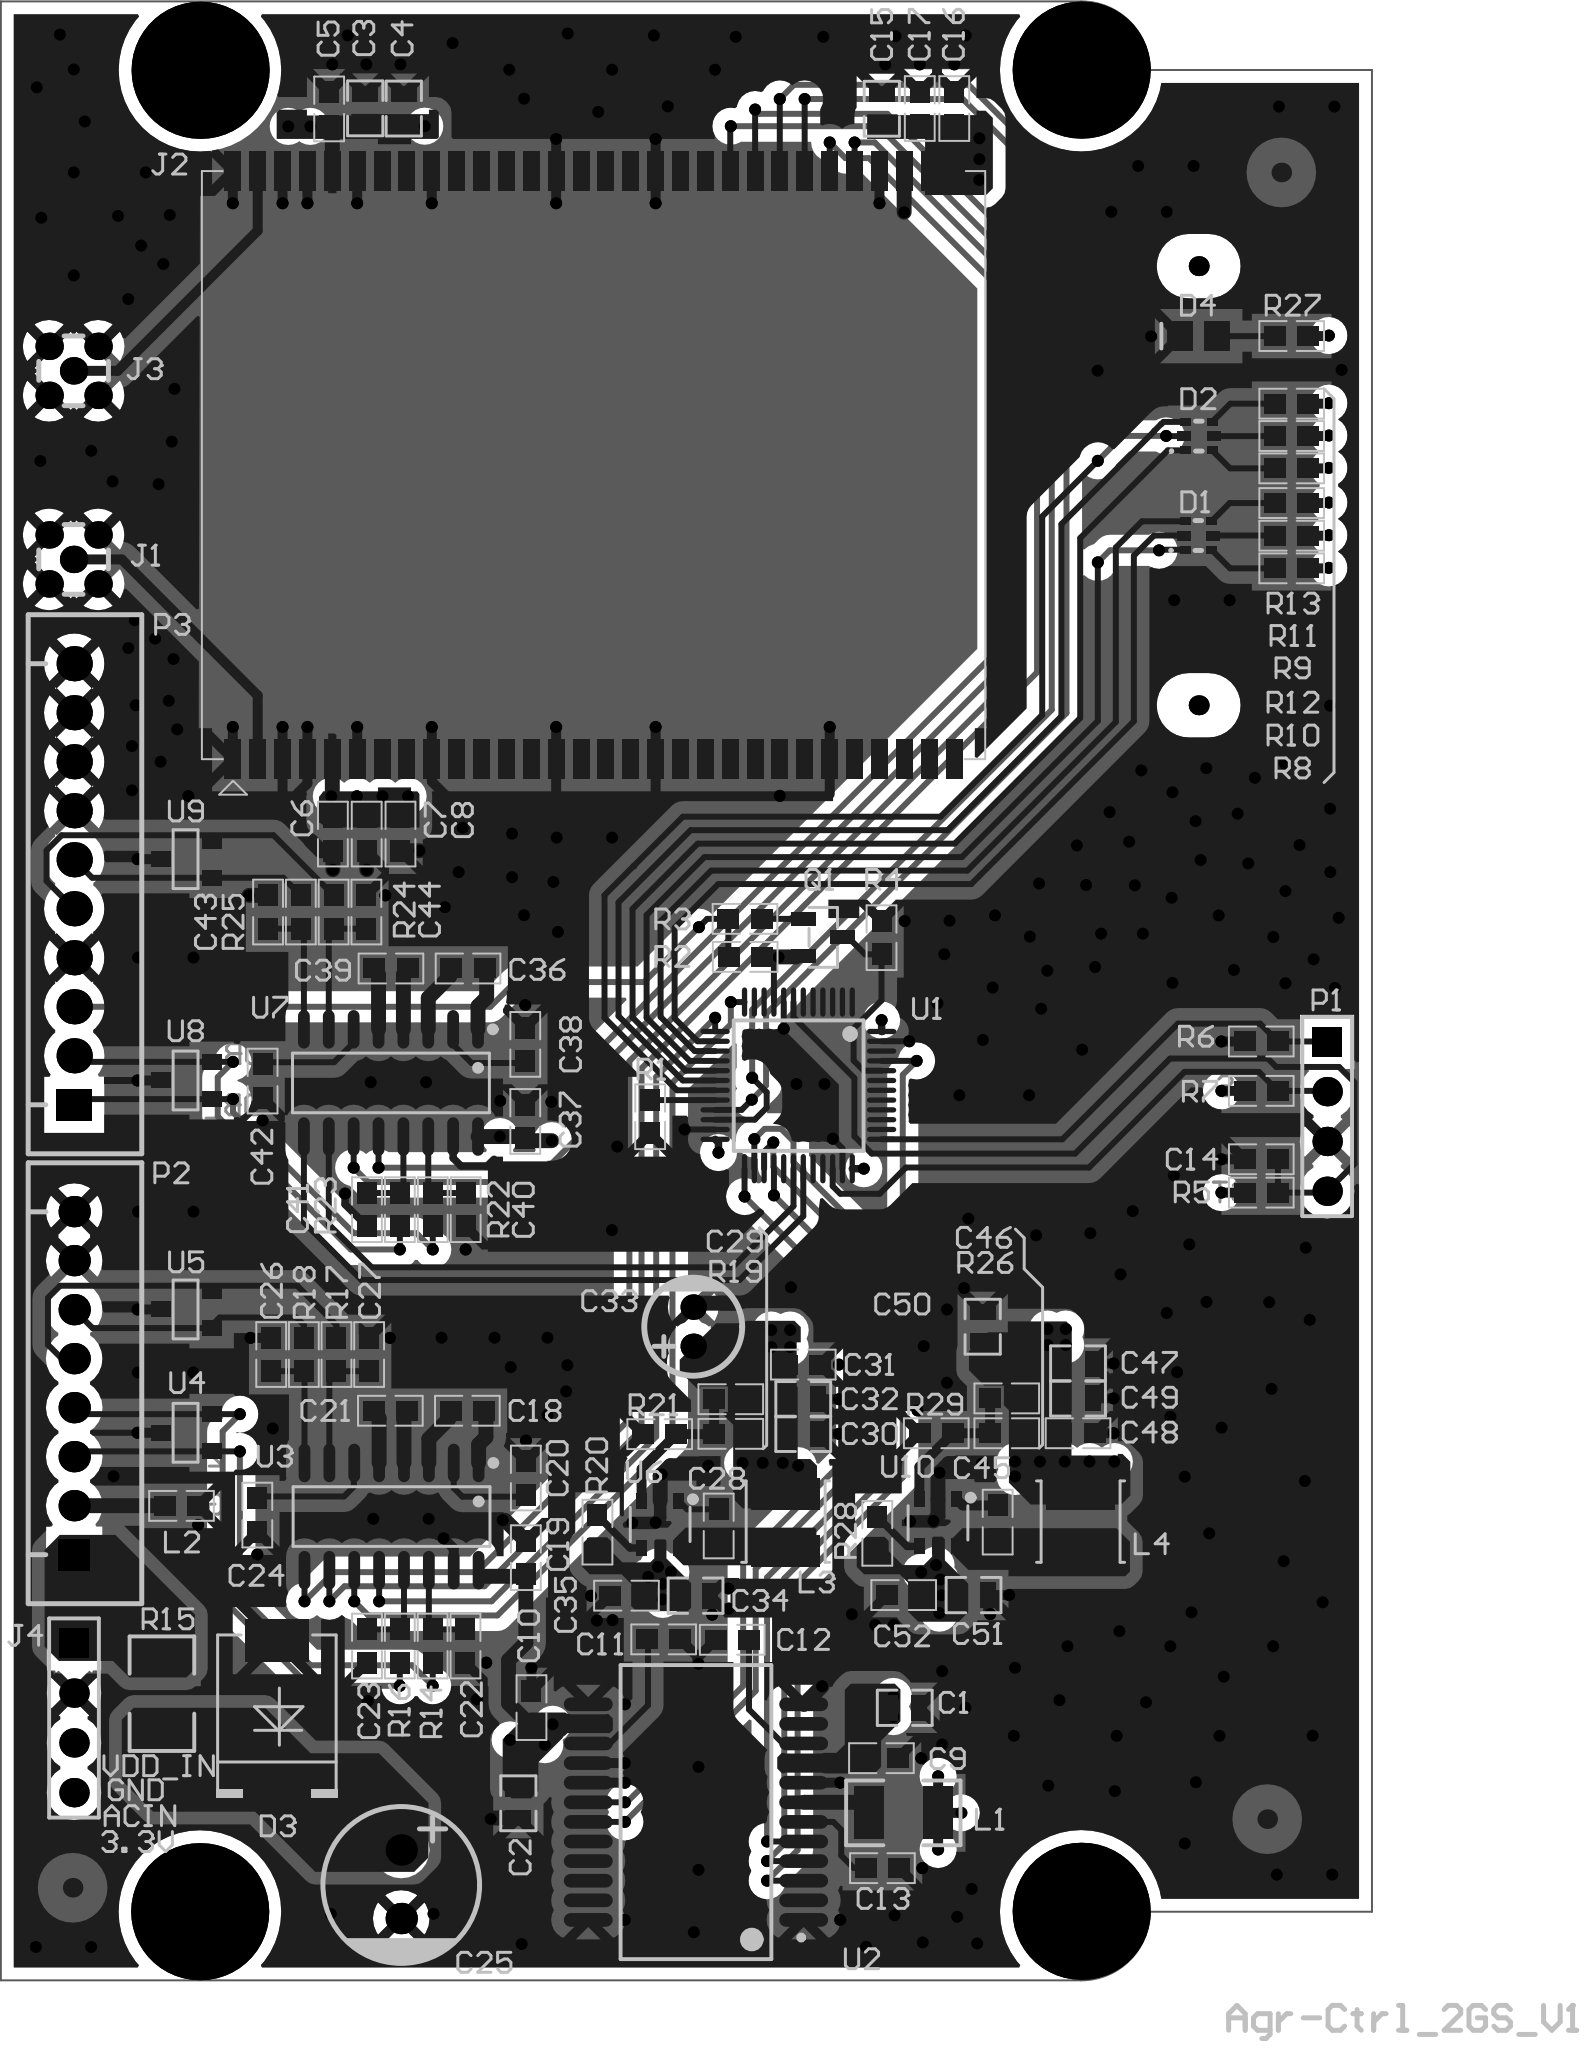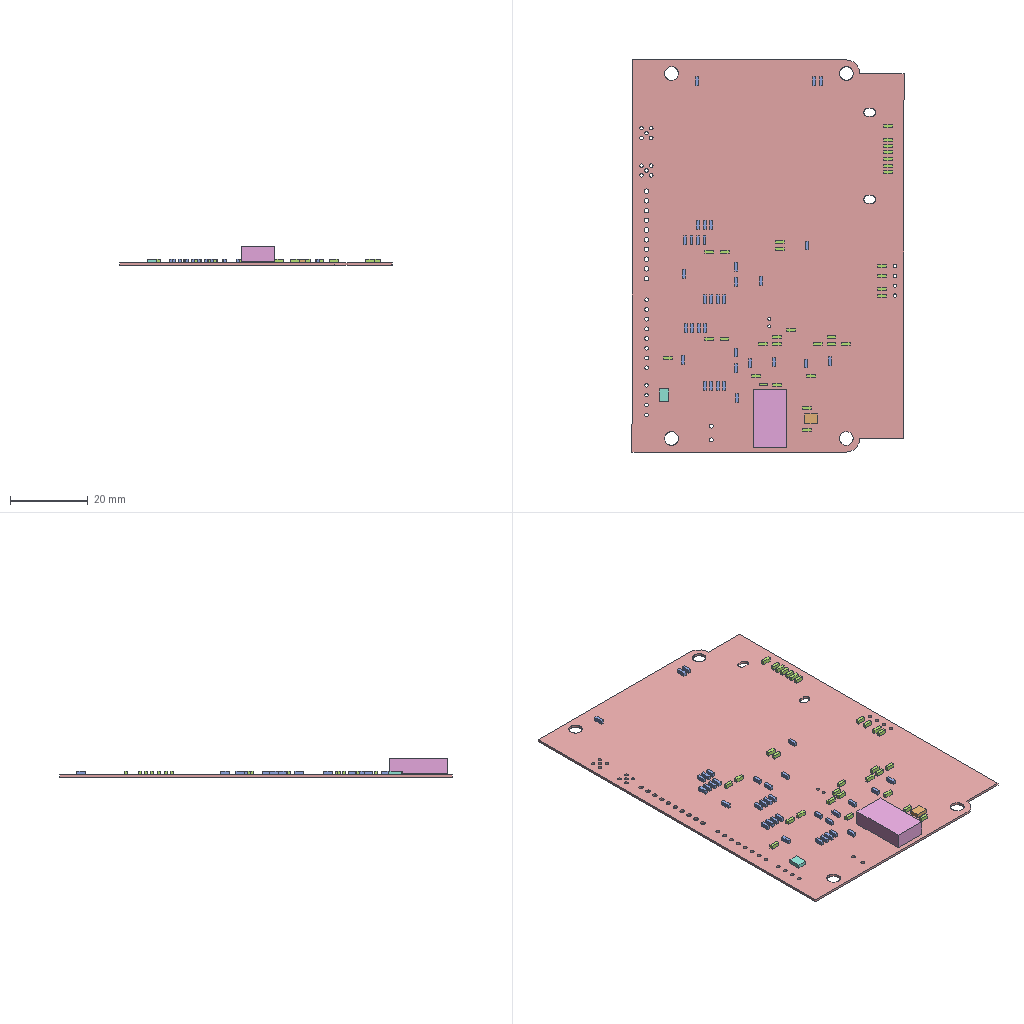Circuit board layout | Altium Designer | box 70 x 100.9 x 4.8 mm
Layer stack:
# Altium Designer layer stack of  (unit mm; dielectric type: 0 none, 1 core, 2 prepreg, 3 surface material)
index,name,kind,layer,copper_thickness_mm,dielectric_type,dielectric_thickness_mm,dielectric_material,dielectric_constant
0,Top Paste,other,,,,,,
1,Top Overlay,other,,,,,,
2,Top Solder,dielectric,,,3,0.0102,Solder Resist,3.5
3,Top Layer,copper,Top Layer,0.0356,,,,
4,Dielectric1,dielectric,,,2,0.0711,PP-006,4.1
5,GND2,copper,GND2,0.035,,,,
6,Dielectric5,dielectric,,,0,0.32,FR-4,4.8
7,POWER3,copper,POWER3,0.035,,,,
8,Dielectric6,dielectric,,,2,0.0711,PP-006,4.1
9,Bottom Layer,copper,Bottom Layer,0.0356,,,,
10,Bottom Solder,dielectric,,,3,0.0102,Solder Resist,3.5
11,Bottom Overlay,other,,,,,,
12,Bottom Paste,other,,,,,,
# drill layer pairs: low layer,high layer
drill_pair,Top Layer,Bottom Layer
Part placement:
Designator,Comment,Layer,Footprint,Center-X(mm),Center-Y(mm),Rotation
U5,PESD15VL2BT,TopLayer,SOT-23,78.797,84,90
P1,Header,TopLayer,HDR1X4,137.06,93.84,270
U7,SP3232EEN,TopLayer,SOP16-6.6,89.255,95.555,270
C41,15pF/50V,TopLayer,0603,88.029,89.09,90
R25,4.7O,±1%,TopLayer,0603,84.653,104.273,270
R24,4.7O,±1%,TopLayer,0603,86.327,104.273,270
R23,4.7O,±1%,TopLayer,0603,89.71,89.09,90
R22,4.7O,±1%,TopLayer,0603,91.39,89.09,90
R21,10K,TopLayer,0603,102.978,77.639,360
R20,100K,TopLayer,0603,99.8,72.64,270
R19,75K 1%,TopLayer,0603,106.608,77.655,360
R18,4.7O,±1%,TopLayer,0603,84.807,81.7,270
R6,10K,TopLayer,0603,133.696,97.67,180
D3,SMCJ18A,TopLayer,SMC_L6.9-W5.9-LS7.9-RD,83.43,63.42,90
C1,22uF/10V,TopLayer,C0805,115.49,63.68,360
C2,22uF/10V,TopLayer,C0805,95.76,58.809,270
C3,10uF/25V,TopLayer,C0805,87.94,145.27,270
C4,10uF/25V,TopLayer,C0805,89.91,145.26,270
C5,100nF/50V,TopLayer,0603,86.1,145.24,90
C6,100pF/50V,TopLayer,0603,86.29,108.25,270
C7,100pF/50V,TopLayer,0603,88.016,108.25,90
C8,100nF/50V,TopLayer,0603,89.741,108.25,90
C9,1uF/25V,TopLayer,0603,114.3,61.11,360
C10,100nF/50V,TopLayer,0603,96.43,63.69,90
C11,1uF/25V,TopLayer,0603,103.18,67.17,360
C12,1uF/25V,TopLayer,0603,106.68,67.15,180
C13,470nF/50V,TopLayer,0603,114.35,55.5,360
C15,10uF/25V,TopLayer,C0805,114.32,145.25,270
C16,100pF/50V,TopLayer,0603,118.02,145.26,270
C17,100nF/50V,TopLayer,0603,116.257,145.26,270
C25,470uF/25V,TopLayer,CAP-TH_BD8.0-P3.50-D1.0-FD,89.78,54.68,270
C28,100nF/50V,TopLayer,0603,105.99,72.956,90
C29,100pF/50V,TopLayer,0603,106.608,79.421,180
C30,22uF/10V,TopLayer,C0805,110.308,77.655,360
C31,100nF/50V,TopLayer,0603,110.308,81.186,360
C32,22uF/10V,TopLayer,C0805,110.308,79.421,360
C33,100uF/10V,TopLayer,CAP-TH_BD5.0-P2.00-D0.8-FD,104.69,83.12,90
C34,10uF/25V,TopLayer,C0805,104.808,69.4,180
C35,100nF/50V,TopLayer,0603,101.28,69.4,360
C39,100nF/50V,TopLayer,0603,89.255,101.392,360
C45,100nF/50V,TopLayer,0603,120.236,73.152,90
C46,100pF/50V,TopLayer,0603,120.7,79.463,180
C47,22uF/10V,TopLayer,C0805,124.339,81.241,360
C48,100nF/50V,TopLayer,0603,124.339,77.685,360
C49,22uF/10V,TopLayer,C0805,124.339,79.463,360
C50,22uF/10V,TopLayer,C0805,119.47,83.12,90
C51,10uF/25V,TopLayer,C0805,119.004,69.43,180
C52,100nF/50V,TopLayer,0603,115.437,69.43,360
D1,Full-color RGB LED,TopLayer,RGB,130.48,123.48,180
D2,Full-color RGB LED,TopLayer,RGB,130.51,128.55,180
D4,RED,TopLayer,LED_0805,130.5,133.65,180
J2,UM482/K823,TopLayer,UM482/K823,99.595,127.07,90
L2,120O ±25% @100MHz,TopLayer,0603,78.56,73.98,360
L3,2.2uH/2A,TopLayer,IND-SMD_L4.0-W4.0,109.41,73.15,90
L4,2.2uH/2A,TopLayer,IND-SMD_L4.0-W4.0,124.47,73.15,90
P2,XH-8A,TopLayer,CONN-TH_XH-8A,73.08,80.24,90
P3,XH-10A,TopLayer,CONN-TH_10P-P2.50_XH-10A,73.08,105.69,90
Q1,8550,TopLayer,SOT-23-SS8550,111.33,102.98,180
R11,680R,TopLayer,0603,135.25,128.555,180
R12,1K,TopLayer,0603,135.25,125.135,180
R13,1K,TopLayer,0603,135.25,130.205,180
R26,100K,TopLayer,0603,120.7,77.685,360
R27,1K,TopLayer,0603,135.25,133.655,360
R28,100K,TopLayer,0603,114.09,72.58,270
R29,22.1K,TopLayer,0603,117.1,77.685,360
U1,STM32F103C8T6/GD32F103C8T6,TopLayer,LQFP-48_L7.0-W7.0-P0.50-LS9.0-BL,110.06,95.43,180
U2,SCC2130,TopLayer,SCC2130D,104.83,58.36,180
U3,SP3232EEN,TopLayer,SOP16-6.6,89.285,73.436,270
U4,PESD15VL2BT,TopLayer,SOT-23,78.797,77.71,90
U8,PESD15VL2BT,TopLayer,SOT-23,78.797,95.68,90
U9,PESD15VL2BT,TopLayer,SOT-23,78.797,106.97,90
R1,10K,TopLayer,0603,102.49,93.83,90
R2,10K,TopLayer,0603,107.344,101.984,360
R4,10K,TopLayer,0603,114.304,102.964,270
R5,10K,TopLayer,0603,133.696,89.96,180
R7,10K,TopLayer,0603,133.696,95.15,180
R8,1.5K,TopLayer,0603,135.25,121.805,180
R9,1.5K,TopLayer,0603,135.25,126.905,180
R10,680R,TopLayer,0603,135.25,123.47,180
R14,4.7O,±1%,TopLayer,0603,91.383,66.831,90
R15,12V/2A,TopLayer,1210,77.56,64.4,90
R16,4.7O,±1%,TopLayer,0603,89.707,66.831,90
R17,4.7O,±1%,TopLayer,0603,86.473,81.7,270
C18,100nF/50V,TopLayer,0603,93.156,78.833,360
C19,100nF/50V,TopLayer,0603,96.143,71.338,90
C20,100nF/50V,TopLayer,0603,96.143,75.401,90
C21,100nF/50V,TopLayer,0603,89.224,78.833,360
C22,15pF/50V,TopLayer,0603,93.06,66.831,90
C23,15pF/50V,TopLayer,0603,88.03,66.831,90
C24,100nF/50V,TopLayer,0603,82.431,73.511,270
C26,15pF/50V,TopLayer,0603,83.14,81.7,90
C27,15pF/50V,TopLayer,0603,88.14,81.7,90
C36,100nF/50V,TopLayer,0603,93.192,101.392,360
C37,100nF/50V,TopLayer,0603,96.113,93.59,90
C38,100nF/50V,TopLayer,0603,96.113,97.522,90
C40,15pF/50V,TopLayer,0603,93.07,89.09,90
C42,100nF/50V,TopLayer,0603,82.7,95.65,270
C43,15pF/50V,TopLayer,0603,82.98,104.273,90
C44,15pF/50V,TopLayer,0603,88,104.273,90
C14,100nF/50V,TopLayer,0603,133.696,91.66,360
L1,47uH±20%,TopLayer,1210,115.418,58.32,180
R3,10K,TopLayer,0603,107.334,103.924,180
J1,MMCX-KE RF connector,TopLayer,MMCX-TH_ZC11.801KK,73.05,122.26,180
J3,MMCX-KE RF connector,TopLayer,MMCX-TH_ZC11.801KK,73.05,131.88,360
J4,Header,TopLayer,HDR1X4,73.07,63.16,270
U6,SY8113B,TopLayer,TSOT-23-6_L2.9-W1.6-P0.95-LS2.8-BR,103.002,73.033,90
U10,SY8113B,TopLayer,TSOT-23-6_L2.9-W1.6-P0.95-LS2.8-BR,117.188,73.113,90
Pad and via stacks:
# Altium Designer via and pad stacks of  (unit mm). Each distinct definition once, with the count of objects using it.
# via: kind,start_layer,end_layer,hole_mm,diameter_mm,mode(0 simple;1 top-mid-bottom;2 full stack),diameter_per_layer,count,example_net
# pad: kind,layer,hole_mm,hole_type(0 round;1 square;2 slot),plating,top_size,top_shape(1 round;2 rect;3 octagon;9 rounded rect),mid_size,bottom_size,mode,footprint,size_per_layer,count,example
pad,Top Layer,0,0,plated,0.8x1,2,0.8x1,0.8x1,0,SOT-23,,12,U9.2
pad,Top Layer,0,0,plated,1.6x3.5,2,1.6x3.5,1.6x3.5,0,IND-SMD_L4.0-W4.0,,4,L4.2
pad,Top Layer,0,0,plated,1.3x0.8,2,1.3x0.8,1.3x0.8,0,C0805,,24,C2.2
pad,Top Layer,0,0,plated,1x1.1,2,1x1.1,1x1.1,0,0603,,134,C42.2
pad,Top Layer,0,0,plated,2.158x3.24,2,2.158x3.24,2.158x3.24,0,SMC_L6.9-W5.9-LS7.9-RD,,2,D3.2
pad,Top Layer,0,0,plated,0.8x0.532,2,0.8x0.532,0.8x0.532,0,TSOT-23-6_L2.9-W1.6-P0.95-LS2.8-BR,,12,U10.1
pad,Top Layer,0,0,plated,1.25x0.7,2,1.25x0.7,1.25x0.7,0,SOT-23-SS8550,,3,Q1.1
pad,Top Layer,0,0,plated,1x1,1,1x1,1x1,0,,,3,MARK
pad,Top Layer,0,0,plated,2.01x0.85,2,2.01x0.85,2.01x0.85,0,UM482/K823,,60,J2.30
pad,Top Layer,0,0,plated,0.602x1.971,1,0.602x1.971,0.602x1.971,0,SOP16-6.6,,32,U7.9
pad,Top Layer,0,0,plated,1.524x2.7,2,1.524x2.7,1.524x2.7,0,1210,,4,L1.1
pad,Top Layer,0,0,plated,0.7x2.5,1,0.7x2.5,0.7x2.5,0,SCC2130D,,24,U2.13
pad,Top Layer,0,0,plated,0.27x1.5,1,0.27x1.5,0.27x1.5,0,LQFP-48_L7.0-W7.0-P0.50-LS9.0-BL,,24,U1.1
pad,Top Layer,0,0,plated,1.5x0.27,1,1.5x0.27,1.5x0.27,0,LQFP-48_L7.0-W7.0-P0.50-LS9.0-BL,,24,U1.13
pad,Top Layer,0,0,plated,0.55x0.4,2,0.55x0.4,0.55x0.4,0,RGB,,8,D1.1
pad,Top Layer,0,0,plated,0.7x0.5,2,0.7x0.5,0.7x0.5,0,RGB,,4,D1.3
pad,Top Layer,0,0,plated,1.5x1.3,2,1.5x1.3,1.5x1.3,0,LED_0805,,2,D4.2
pad,Multi-Layer,0.8,0,plated,1.3x1.3,1,1.3x1.3,1.3x1.3,0,CAP-TH_BD5.0-P2.00-D0.8-FD,,2,C33.1
pad,Multi-Layer,2,2,unplated,1.016x1.016,1,1.016x1.016,1.016x1.016,0,,,2,0
pad,Multi-Layer,0.9,0,plated,1.5x1.5,2,1.5x1.5,1.5x1.5,0,HDR1X4,,2,P1.1
pad,Multi-Layer,0.9,0,plated,1.5x1.5,1,1.5x1.5,1.5x1.5,0,HDR1X4,,6,P1.2
pad,Multi-Layer,1,0,plated,1.6x1.6,1,1.6x1.6,1.6x1.6,0,CAP-TH_BD8.0-P3.50-D1.0-FD,,2,C25.2
pad,Multi-Layer,0.9,0,plated,1.4x1.4,1,1.4x1.4,1.4x1.4,0,MMCX-TH_ZC11.801KK,,10,J3.5
pad,Multi-Layer,1.2,0,plated,1.8x1.8,1,1.8x1.8,1.8x1.8,0,CONN-TH_10P-P2.50_XH-10A,,9,P3.10
pad,Multi-Layer,1.2,0,plated,1.6x1.8,2,1.6x1.8,1.6x1.8,0,CONN-TH_10P-P2.50_XH-10A,,1,P3.1
pad,Multi-Layer,1,0,plated,1.6x1.6,1,1.6x1.6,1.6x1.6,0,CONN-TH_XH-8A,,7,P2.8
pad,Multi-Layer,1,0,plated,1.6x1.6,2,1.6x1.6,1.6x1.6,0,CONN-TH_XH-8A,,1,P2.1
pad,Multi-Layer,3.5,0,unplated,7x7,1,7x7,7x7,0,,,4,1
via,Top Layer,Bottom Layer,0.3048,0.6096,0,,390,GND
Copper pours:
name,layer,net,type(0 solid;1 hatched;2 none)
BottomLayer-No Net,Top Layer,VDD_12V,0
BottomLayer-No Net,Top Layer,VDD_12V,0
BottomLayer-No Net,Top Layer,VDD_12V,0
BottomLayer-No Net,Top Layer,VDD_IN,0
Top Layer-GND 1,Top Layer,GND,0
Top Layer-VDD_3.3,Top Layer,VDD_3.3,0
Top Layer-GND,Top Layer,GND,0
Top Layer-GND,Top Layer,GND,0
Top Layer-VDD_5V,Top Layer,VDD_5V,0
Top Layer-VDD_3.3 3,Top Layer,VDD_3.3,0
Top Layer-VDD_5V 1,Top Layer,VDD_5V,0
Top Layer-VDD_3.3 1,Top Layer,VDD_3.3,0
Top Layer-VDD_3.3 2,Top Layer,VDD_3.3,0
Top Layer-VDD_5V 2,Top Layer,VDD_5V,0
Top Layer-NetC45_1,Top Layer,NetC45_1,0
Top Layer-NetC28_1,Top Layer,NetC28_1,0
Bottom Layer-GND,Bottom Layer,GND,0
Design rules, without the lines most boards share:
# Altium Designer design rules of  (exported by Altium Designer, unit mm)
# columns: name | kind | enabled | priority | scope1 | scope2 | descriptor | typed fields (field=value)
PolygonConnect_1 | 20 | enabled | 1 | ISVIA | All | Polygon Connect Rule(Direct Connect )(Conductor Width=10mil) (Relief Angle=90 Angle) (Entries=4) (Air Gap Width=10mil) (ISVIA),(All) | connect_style(0=relief,1=direct,2=none)=1 relief_conductor_width=0.254 relief_entries=4
Clearance | 0 | enabled | 3 | All | All | Clearance Constraint (Gap=6mil) (All),(All) | gap=0.1524
mark | 0 | enabled | 1 | HASPAD('FREE-MARK') | All | Clearance Constraint (Gap=50mil) (HASPAD('FREE-MARK')),(All) | gap=1.27
PolygonConnect | 20 | enabled | 3 | All | All | Polygon Connect Rule(Direct Connect )(Conductor Width=10mil) (Relief Angle=90 Angle) (Entries=4) (Air Gap Width=10mil) (All),(All) | connect_style(0=relief,1=direct,2=none)=1 relief_conductor_width=0.254 relief_entries=4
PolygonGND | 20 | enabled | 2 | InNet('GND') | All | Polygon Connect Rule(Relief Connect )(Conductor Width=20mil) (Relief Angle=45 Angle) (Entries=4) (Air Gap Width=10mil) (InNet('GND')),(All) | connect_style(0=relief,1=direct,2=none)=0 relief_conductor_width=0.508 relief_entries=4
GND_Clearance | 0 | enabled | 2 | InNet('GND') | All | Clearance Constraint (Gap=6mil) (InNet('GND')),(All) | gap=0.1524
PlaneConnect | 6 | enabled | 1 | All | All | Power Plane Connect Rule(Direct Connect )(Expansion=15mil) (Conductor Width=15mil) (Air Gap=15mil) (Entries=4) (All) | relief_conductor_width=0.381 relief_entries=4 relief_expansion=0.381
PlaneClearance | 12 | enabled | 1 | All | All | Power Plane Clearance (Clearance =25mil) (All) | clearance=0.635
Width | 2 | enabled | 1 | All | All | Width Constraint (Min=6mil) (Max=30mil) (Preferred=10mil) (All) |
RoutingVias | 11 | enabled | 1 | All | All | Routing Via (MinHoleWidth=12mil) (MaxHoleWidth=12mil) (PreferredHoleWidth=12mil) (MinWidth=24mil) (MaxWidth=24mil) (PreferedWidth=24mil) (All) | via_min_hole=0.3048 via_max_hole=0.3048 via_preferred_diameter=0.6096 via_preferred_hole=0.3048
PasteMaskExpansion | 14 | enabled | 1 | All | All | Paste Mask Expansion (Expansion =0mil) (All) | expansion=0
SolderMaskExpansion | 13 | enabled | 1 | All | All | Solder Mask Expansion (Expansion =2.5mil) (All) | expansion=0.0635
ComponentClearance | 24 | enabled | 1 | All | All | Component Clearance Constraint ( Horizontal Gap = 0mil, Vertical Gap = 0mil ) (All),(All)  | gap=0
HoleSize | 42 | enabled | 1 | All | All | Hole Size Constraint (Min=12mil) (Max=500mil) (All) |
DiffPairsRouting | 51 | enabled | 1 | All | All | Differential Pairs Uncoupled Length using the Gap Constraints (Min=10mil) (Max=10mil) (Prefered=10mil)  and Width Constraints (Min=15mil) (Max=15mil) (Prefered=15mil) (All) |
HoleToHoleClearance | 52 | enabled | 1 | All | All | Hole To Hole Clearance (Gap=0mil) (All),(All) | gap=0
MinimumSolderMaskSliver | 53 | enabled | 1 | All | All | Minimum Solder Mask Sliver (Gap=0mil) (All),(All) |
SilkToSolderMaskClearance | 54 | enabled | 1 | IsPad | All | Silk To Solder Mask (Clearance=0mil) (IsPad),(All) |
SilkToSilkClearance | 55 | enabled | 1 | All | All | Silk to Silk (Clearance=0mil) (All),(All) |
Classes set for this board:
# Altium Designer classes of  (member kind: 0 net, 1 component, 2 from-to, 3 pad, 4 layer, 5 differential pair, 6 design channel, 7 polygon, 8 structure, 9 xSignal)
# columns: class name | member kind | superclass | members
Agr-Ctrl-2GS_v1.1 | 1 | no | C1; C2; C3; C4; C5; C6; C7; C8; C9; C10; C11; C12; C13; C14; C15; C16; C17; C18; C19; C20; C21; C22; C23; C24; C25; C26; C27; C28; C29; C30; C31; C32; C33; C34; C35; C36; C37; C38; C39; C40; C42; C43; C44; C45; C46; C47; C48; C49; C50; C51; C52; D1; D2; J1; J2; J3; J4; L1; L2; L3; Q1; R1; R7; R8; R9; R10; R11; R12; R13; R14; R15; R16; R17; U1; U2; U3; U4; U6; U8; U9; U10; R1; R7; R8; R9; R10; R14; R15; R16; R17; C18; C19; C20; C21; C22; C23; C24; C26; C27; C36; C37; C38; C40; C42; C43; C44; C14; L1; J1; J3; J4; U6; U10; R22; R23; R24; R25; D4; P3; R26; R27; R28; R29; D4; R27; P3; R3; R29; R26; P2; R4; R28; D3; L4; R2; R5; R6; R18; R19; R20; R21; C41; P1; U7; U5;